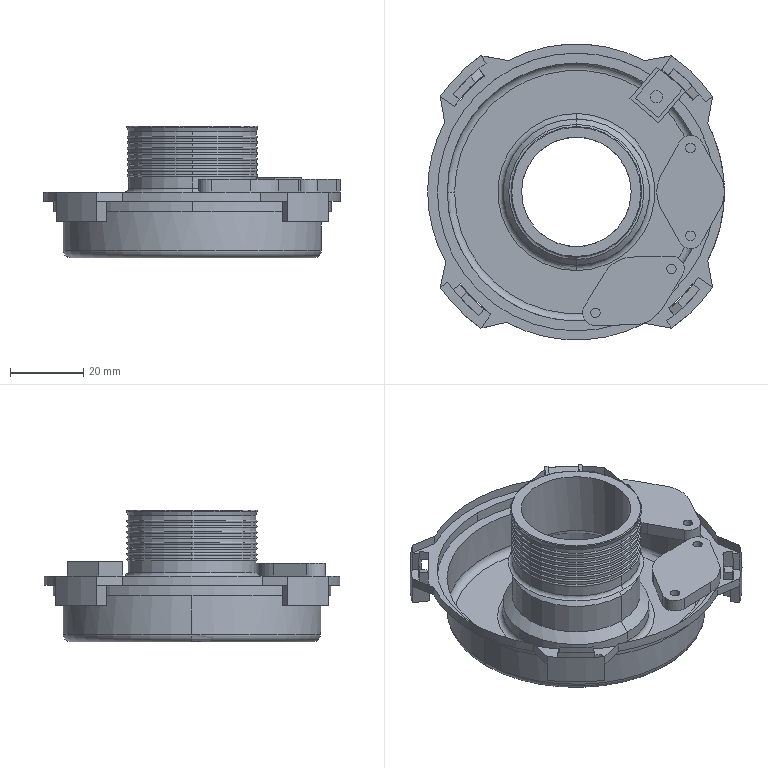Part | STEP file | ZHULVGAI_18_1_1_1 | 1 solid | 164 faces | box 81.19 x 81 x 36 mm | volume 66134 mm3 | plane 68 | cylinder 66 | torus 24 | cone 6 | commonest cylinder face diameters 35 x20 2.6 x8 81 x8 7 x4 18.5 x4 81.5 x4